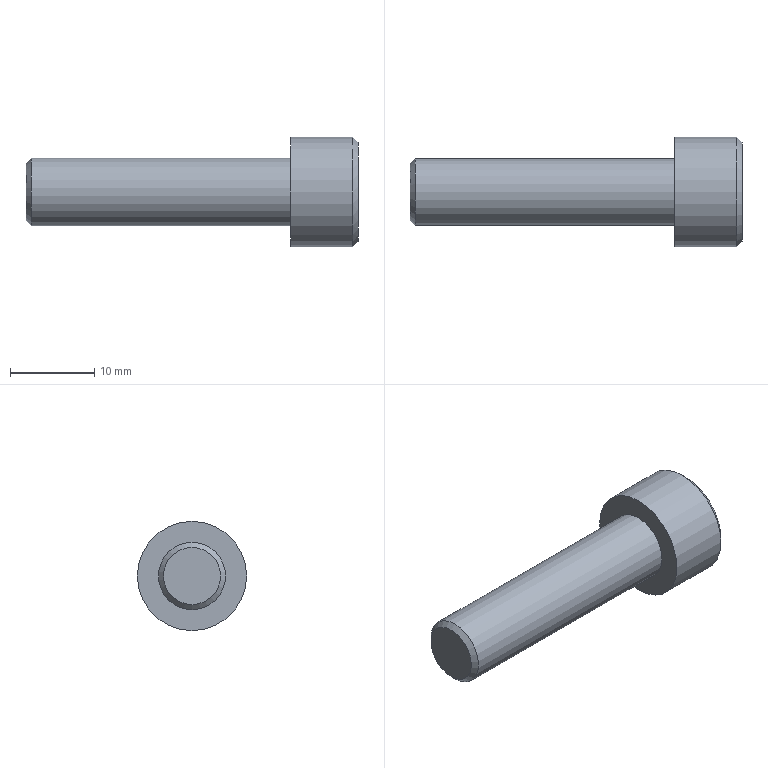Part | NX | features M8.00-60.00 2 | 1 solid | 14 faces | box 39.5 x 13 x 13 mm | volume 2474 mm3 | plane 10 | cylinder 2 | cone 2 | commonest cylinder face diameters 8 x1 13 x1
STEP:
#1=CARTESIAN_POINT('',(103.775,14.,24.349));
#2=VERTEX_POINT('',#1);
#3=CARTESIAN_POINT('',(103.775,14.,18.449));
#4=DIRECTION('',(1.,0.,0.));
#5=DIRECTION('',(0.,0.,1.));
#6=AXIS2_PLACEMENT_3D('',#3,#4,#5);
#7=CIRCLE('',#6,5.9);
#8=EDGE_CURVE('',#2,#2,#7,.T.);
#9=ORIENTED_EDGE('',*,*,#8,.T.);
#10=EDGE_LOOP('',(#9));
#11=FACE_BOUND('',#10,.T.);
#12=CARTESIAN_POINT('',(103.775,17.4,16.486));
#13=VERTEX_POINT('',#12);
#14=CARTESIAN_POINT('',(103.775,17.4,20.412));
#15=VERTEX_POINT('',#14);
#16=CARTESIAN_POINT('',(103.775,17.4,16.486));
#17=DIRECTION('',(0.,0.,1.));
#18=VECTOR('',#17,1000.);
#19=LINE('',#16,#18);
#20=EDGE_CURVE('',#13,#15,#19,.T.);
#21=ORIENTED_EDGE('',*,*,#20,.F.);
#22=CARTESIAN_POINT('',(103.775,14.,14.523));
#23=VERTEX_POINT('',#22);
#24=CARTESIAN_POINT('',(103.775,14.,14.523));
#25=DIRECTION('',(0.,0.866,0.5));
#26=VECTOR('',#25,1000.);
#27=LINE('',#24,#26);
#28=EDGE_CURVE('',#23,#13,#27,.T.);
#29=ORIENTED_EDGE('',*,*,#28,.F.);
#30=CARTESIAN_POINT('',(103.775,10.6,16.486));
#31=VERTEX_POINT('',#30);
#32=CARTESIAN_POINT('',(103.775,10.6,16.486));
#33=DIRECTION('',(0.,0.866,-0.5));
#34=VECTOR('',#33,1000.);
#35=LINE('',#32,#34);
#36=EDGE_CURVE('',#31,#23,#35,.T.);
#37=ORIENTED_EDGE('',*,*,#36,.F.);
#38=CARTESIAN_POINT('',(103.775,10.6,20.412));
#39=VERTEX_POINT('',#38);
#40=CARTESIAN_POINT('',(103.775,10.6,20.412));
#41=DIRECTION('',(0.,0.,-1.));
#42=VECTOR('',#41,1000.);
#43=LINE('',#40,#42);
#44=EDGE_CURVE('',#39,#31,#43,.T.);
#45=ORIENTED_EDGE('',*,*,#44,.F.);
#46=CARTESIAN_POINT('',(103.775,14.,22.375));
#47=VERTEX_POINT('',#46);
#48=CARTESIAN_POINT('',(103.775,14.,22.375));
#49=DIRECTION('',(0.,-0.866,-0.5));
#50=VECTOR('',#49,1000.);
#51=LINE('',#48,#50);
#52=EDGE_CURVE('',#47,#39,#51,.T.);
#53=ORIENTED_EDGE('',*,*,#52,.F.);
#54=CARTESIAN_POINT('',(103.775,17.4,20.412));
#55=DIRECTION('',(0.,-0.866,0.5));
#56=VECTOR('',#55,1000.);
#57=LINE('',#54,#56);
#58=EDGE_CURVE('',#15,#47,#57,.T.);
#59=ORIENTED_EDGE('',*,*,#58,.F.);
#60=EDGE_LOOP('',(#21,#29,#37,#45,#53,#59));
#61=FACE_BOUND('',#60,.T.);
#62=CARTESIAN_POINT('',(103.775,14.,18.449));
#63=DIRECTION('',(1.,0.,0.));
#64=DIRECTION('',(0.,0.,1.));
#65=AXIS2_PLACEMENT_3D('',#62,#63,#64);
#66=PLANE('',#65);
#67=ADVANCED_FACE('',(#11,#61),#66,.T.);
#68=CARTESIAN_POINT('',(95.775,14.,14.449));
#69=VERTEX_POINT('',#68);
#70=CARTESIAN_POINT('',(95.775,14.,18.449));
#71=DIRECTION('',(-1.,0.,0.));
#72=DIRECTION('',(0.,0.,-1.));
#73=AXIS2_PLACEMENT_3D('',#70,#71,#72);
#74=CIRCLE('',#73,4.);
#75=EDGE_CURVE('',#69,#69,#74,.T.);
#76=ORIENTED_EDGE('',*,*,#75,.F.);
#77=EDGE_LOOP('',(#76));
#78=FACE_BOUND('',#77,.T.);
#79=CARTESIAN_POINT('',(95.775,14.,24.949));
#80=VERTEX_POINT('',#79);
#81=CARTESIAN_POINT('',(95.775,14.,18.449));
#82=DIRECTION('',(1.,0.,0.));
#83=DIRECTION('',(0.,0.,1.));
#84=AXIS2_PLACEMENT_3D('',#81,#82,#83);
#85=CIRCLE('',#84,6.5);
#86=EDGE_CURVE('',#80,#80,#85,.T.);
#87=ORIENTED_EDGE('',*,*,#86,.F.);
#88=EDGE_LOOP('',(#87));
#89=FACE_BOUND('',#88,.T.);
#90=CARTESIAN_POINT('',(95.775,14.,18.449));
#91=DIRECTION('',(-1.,0.,0.));
#92=DIRECTION('',(0.,0.,-1.));
#93=AXIS2_PLACEMENT_3D('',#90,#91,#92);
#94=PLANE('',#93);
#95=ADVANCED_FACE('',(#78,#89),#94,.T.);
#96=CARTESIAN_POINT('',(103.175,14.,24.949));
#97=VERTEX_POINT('',#96);
#98=CARTESIAN_POINT('',(103.175,14.,18.449));
#99=DIRECTION('',(1.,0.,0.));
#100=DIRECTION('',(0.,0.,1.));
#101=AXIS2_PLACEMENT_3D('',#98,#99,#100);
#102=CIRCLE('',#101,6.5);
#103=EDGE_CURVE('',#97,#97,#102,.F.);
#104=ORIENTED_EDGE('',*,*,#103,.T.);
#105=EDGE_LOOP('',(#104));
#106=FACE_BOUND('',#105,.T.);
#107=ORIENTED_EDGE('',*,*,#86,.T.);
#108=EDGE_LOOP('',(#107));
#109=FACE_BOUND('',#108,.T.);
#110=CARTESIAN_POINT('',(95.775,14.,18.449));
#111=DIRECTION('',(1.,0.,0.));
#112=DIRECTION('',(0.,0.,1.));
#113=AXIS2_PLACEMENT_3D('',#110,#111,#112);
#114=CYLINDRICAL_SURFACE('',#113,6.5);
#115=ADVANCED_FACE('',(#106,#109),#114,.T.);
#116=CARTESIAN_POINT('',(64.275,14.,15.049));
#117=VERTEX_POINT('',#116);
#118=CARTESIAN_POINT('',(64.275,14.,18.449));
#119=DIRECTION('',(-1.,0.,0.));
#120=DIRECTION('',(0.,0.,-1.));
#121=AXIS2_PLACEMENT_3D('',#118,#119,#120);
#122=CIRCLE('',#121,3.4);
#123=EDGE_CURVE('',#117,#117,#122,.T.);
#124=ORIENTED_EDGE('',*,*,#123,.T.);
#125=EDGE_LOOP('',(#124));
#126=FACE_BOUND('',#125,.T.);
#127=CARTESIAN_POINT('',(64.275,14.,18.449));
#128=DIRECTION('',(-1.,0.,0.));
#129=DIRECTION('',(0.,0.,-1.));
#130=AXIS2_PLACEMENT_3D('',#127,#128,#129);
#131=PLANE('',#130);
#132=ADVANCED_FACE('',(#126),#131,.T.);
#133=CARTESIAN_POINT('',(64.875,14.,14.449));
#134=VERTEX_POINT('',#133);
#135=CARTESIAN_POINT('',(64.875,14.,18.449));
#136=DIRECTION('',(-1.,0.,0.));
#137=DIRECTION('',(0.,0.,-1.));
#138=AXIS2_PLACEMENT_3D('',#135,#136,#137);
#139=CIRCLE('',#138,4.);
#140=EDGE_CURVE('',#134,#134,#139,.F.);
#141=ORIENTED_EDGE('',*,*,#140,.T.);
#142=EDGE_LOOP('',(#141));
#143=FACE_BOUND('',#142,.T.);
#144=ORIENTED_EDGE('',*,*,#75,.T.);
#145=EDGE_LOOP('',(#144));
#146=FACE_BOUND('',#145,.T.);
#147=CARTESIAN_POINT('',(116.275,14.,18.449));
#148=DIRECTION('',(-1.,0.,0.));
#149=DIRECTION('',(0.,0.,-1.));
#150=AXIS2_PLACEMENT_3D('',#147,#148,#149);
#151=CYLINDRICAL_SURFACE('',#150,4.);
#152=ADVANCED_FACE('',(#143,#146),#151,.T.);
#153=ORIENTED_EDGE('',*,*,#58,.T.);
#154=CARTESIAN_POINT('',(99.775,14.,22.375));
#155=VERTEX_POINT('',#154);
#156=CARTESIAN_POINT('',(99.775,14.,22.375));
#157=DIRECTION('',(1.,0.,0.));
#158=VECTOR('',#157,1000.);
#159=LINE('',#156,#158);
#160=EDGE_CURVE('',#47,#155,#159,.F.);
#161=ORIENTED_EDGE('',*,*,#160,.T.);
#162=CARTESIAN_POINT('',(99.775,17.4,20.412));
#163=VERTEX_POINT('',#162);
#164=CARTESIAN_POINT('',(99.775,17.4,20.412));
#165=DIRECTION('',(0.,-0.866,0.5));
#166=VECTOR('',#165,1000.);
#167=LINE('',#164,#166);
#168=EDGE_CURVE('',#155,#163,#167,.F.);
#169=ORIENTED_EDGE('',*,*,#168,.T.);
#170=CARTESIAN_POINT('',(99.775,17.4,20.412));
#171=DIRECTION('',(1.,0.,0.));
#172=VECTOR('',#171,1000.);
#173=LINE('',#170,#172);
#174=EDGE_CURVE('',#15,#163,#173,.F.);
#175=ORIENTED_EDGE('',*,*,#174,.F.);
#176=EDGE_LOOP('',(#153,#161,#169,#175));
#177=FACE_BOUND('',#176,.T.);
#178=CARTESIAN_POINT('',(101.775,15.7,21.393));
#179=DIRECTION('',(0.,0.5,0.866));
#180=DIRECTION('',(0.,-0.866,0.5));
#181=AXIS2_PLACEMENT_3D('',#178,#179,#180);
#182=PLANE('',#181);
#183=ADVANCED_FACE('',(#177),#182,.F.);
#184=ORIENTED_EDGE('',*,*,#20,.T.);
#185=ORIENTED_EDGE('',*,*,#174,.T.);
#186=CARTESIAN_POINT('',(99.775,17.4,16.486));
#187=VERTEX_POINT('',#186);
#188=CARTESIAN_POINT('',(99.775,17.4,16.486));
#189=DIRECTION('',(0.,0.,1.));
#190=VECTOR('',#189,1000.);
#191=LINE('',#188,#190);
#192=EDGE_CURVE('',#163,#187,#191,.F.);
#193=ORIENTED_EDGE('',*,*,#192,.T.);
#194=CARTESIAN_POINT('',(99.775,17.4,16.486));
#195=DIRECTION('',(1.,0.,0.));
#196=VECTOR('',#195,1000.);
#197=LINE('',#194,#196);
#198=EDGE_CURVE('',#13,#187,#197,.F.);
#199=ORIENTED_EDGE('',*,*,#198,.F.);
#200=EDGE_LOOP('',(#184,#185,#193,#199));
#201=FACE_BOUND('',#200,.T.);
#202=CARTESIAN_POINT('',(101.775,17.4,18.449));
#203=DIRECTION('',(0.,1.,0.));
#204=DIRECTION('',(1.,0.,0.));
#205=AXIS2_PLACEMENT_3D('',#202,#203,#204);
#206=PLANE('',#205);
#207=ADVANCED_FACE('',(#201),#206,.F.);
#208=ORIENTED_EDGE('',*,*,#28,.T.);
#209=ORIENTED_EDGE('',*,*,#198,.T.);
#210=CARTESIAN_POINT('',(99.775,14.,14.523));
#211=VERTEX_POINT('',#210);
#212=CARTESIAN_POINT('',(99.775,14.,14.523));
#213=DIRECTION('',(0.,0.866,0.5));
#214=VECTOR('',#213,1000.);
#215=LINE('',#212,#214);
#216=EDGE_CURVE('',#187,#211,#215,.F.);
#217=ORIENTED_EDGE('',*,*,#216,.T.);
#218=CARTESIAN_POINT('',(99.775,14.,14.523));
#219=DIRECTION('',(1.,0.,0.));
#220=VECTOR('',#219,1000.);
#221=LINE('',#218,#220);
#222=EDGE_CURVE('',#23,#211,#221,.F.);
#223=ORIENTED_EDGE('',*,*,#222,.F.);
#224=EDGE_LOOP('',(#208,#209,#217,#223));
#225=FACE_BOUND('',#224,.T.);
#226=CARTESIAN_POINT('',(101.775,15.7,15.504));
#227=DIRECTION('',(0.,0.5,-0.866));
#228=DIRECTION('',(0.,0.866,0.5));
#229=AXIS2_PLACEMENT_3D('',#226,#227,#228);
#230=PLANE('',#229);
#231=ADVANCED_FACE('',(#225),#230,.F.);
#232=ORIENTED_EDGE('',*,*,#36,.T.);
#233=ORIENTED_EDGE('',*,*,#222,.T.);
#234=CARTESIAN_POINT('',(99.775,10.6,16.486));
#235=VERTEX_POINT('',#234);
#236=CARTESIAN_POINT('',(99.775,10.6,16.486));
#237=DIRECTION('',(0.,0.866,-0.5));
#238=VECTOR('',#237,1000.);
#239=LINE('',#236,#238);
#240=EDGE_CURVE('',#211,#235,#239,.F.);
#241=ORIENTED_EDGE('',*,*,#240,.T.);
#242=CARTESIAN_POINT('',(99.775,10.6,16.486));
#243=DIRECTION('',(1.,0.,0.));
#244=VECTOR('',#243,1000.);
#245=LINE('',#242,#244);
#246=EDGE_CURVE('',#31,#235,#245,.F.);
#247=ORIENTED_EDGE('',*,*,#246,.F.);
#248=EDGE_LOOP('',(#232,#233,#241,#247));
#249=FACE_BOUND('',#248,.T.);
#250=CARTESIAN_POINT('',(101.775,12.3,15.504));
#251=DIRECTION('',(0.,-0.5,-0.866));
#252=DIRECTION('',(0.,0.866,-0.5));
#253=AXIS2_PLACEMENT_3D('',#250,#251,#252);
#254=PLANE('',#253);
#255=ADVANCED_FACE('',(#249),#254,.F.);
#256=ORIENTED_EDGE('',*,*,#44,.T.);
#257=ORIENTED_EDGE('',*,*,#246,.T.);
#258=CARTESIAN_POINT('',(99.775,10.6,20.412));
#259=VERTEX_POINT('',#258);
#260=CARTESIAN_POINT('',(99.775,10.6,20.412));
#261=DIRECTION('',(0.,0.,-1.));
#262=VECTOR('',#261,1000.);
#263=LINE('',#260,#262);
#264=EDGE_CURVE('',#235,#259,#263,.F.);
#265=ORIENTED_EDGE('',*,*,#264,.T.);
#266=CARTESIAN_POINT('',(99.775,10.6,20.412));
#267=DIRECTION('',(1.,0.,0.));
#268=VECTOR('',#267,1000.);
#269=LINE('',#266,#268);
#270=EDGE_CURVE('',#39,#259,#269,.F.);
#271=ORIENTED_EDGE('',*,*,#270,.F.);
#272=EDGE_LOOP('',(#256,#257,#265,#271));
#273=FACE_BOUND('',#272,.T.);
#274=CARTESIAN_POINT('',(101.775,10.6,18.449));
#275=DIRECTION('',(0.,-1.,0.));
#276=DIRECTION('',(-1.,0.,0.));
#277=AXIS2_PLACEMENT_3D('',#274,#275,#276);
#278=PLANE('',#277);
#279=ADVANCED_FACE('',(#273),#278,.F.);
#280=ORIENTED_EDGE('',*,*,#52,.T.);
#281=ORIENTED_EDGE('',*,*,#270,.T.);
#282=CARTESIAN_POINT('',(99.775,14.,22.375));
#283=DIRECTION('',(0.,-0.866,-0.5));
#284=VECTOR('',#283,1000.);
#285=LINE('',#282,#284);
#286=EDGE_CURVE('',#259,#155,#285,.F.);
#287=ORIENTED_EDGE('',*,*,#286,.T.);
#288=ORIENTED_EDGE('',*,*,#160,.F.);
#289=EDGE_LOOP('',(#280,#281,#287,#288));
#290=FACE_BOUND('',#289,.T.);
#291=CARTESIAN_POINT('',(101.775,12.3,21.393));
#292=DIRECTION('',(0.,-0.5,0.866));
#293=DIRECTION('',(0.,-0.866,-0.5));
#294=AXIS2_PLACEMENT_3D('',#291,#292,#293);
#295=PLANE('',#294);
#296=ADVANCED_FACE('',(#290),#295,.F.);
#297=ORIENTED_EDGE('',*,*,#286,.F.);
#298=ORIENTED_EDGE('',*,*,#264,.F.);
#299=ORIENTED_EDGE('',*,*,#240,.F.);
#300=ORIENTED_EDGE('',*,*,#216,.F.);
#301=ORIENTED_EDGE('',*,*,#192,.F.);
#302=ORIENTED_EDGE('',*,*,#168,.F.);
#303=EDGE_LOOP('',(#297,#298,#299,#300,#301,#302));
#304=FACE_BOUND('',#303,.T.);
#305=CARTESIAN_POINT('',(99.775,14.,18.449));
#306=DIRECTION('',(-1.,0.,0.));
#307=DIRECTION('',(0.,0.,-1.));
#308=AXIS2_PLACEMENT_3D('',#305,#306,#307);
#309=PLANE('',#308);
#310=ADVANCED_FACE('',(#304),#309,.F.);
#311=ORIENTED_EDGE('',*,*,#123,.F.);
#312=EDGE_LOOP('',(#311));
#313=FACE_BOUND('',#312,.T.);
#314=ORIENTED_EDGE('',*,*,#140,.F.);
#315=EDGE_LOOP('',(#314));
#316=FACE_BOUND('',#315,.T.);
#317=CARTESIAN_POINT('',(64.875,14.,18.449));
#318=DIRECTION('',(1.,0.,0.));
#319=DIRECTION('',(0.,0.,1.));
#320=AXIS2_PLACEMENT_3D('',#317,#318,#319);
#321=CONICAL_SURFACE('',#320,4.,0.7854);
#322=ADVANCED_FACE('',(#313,#316),#321,.T.);
#323=ORIENTED_EDGE('',*,*,#8,.F.);
#324=EDGE_LOOP('',(#323));
#325=FACE_BOUND('',#324,.T.);
#326=ORIENTED_EDGE('',*,*,#103,.F.);
#327=EDGE_LOOP('',(#326));
#328=FACE_BOUND('',#327,.T.);
#329=CARTESIAN_POINT('',(103.175,14.,18.449));
#330=DIRECTION('',(-1.,0.,0.));
#331=DIRECTION('',(0.,0.,-1.));
#332=AXIS2_PLACEMENT_3D('',#329,#330,#331);
#333=CONICAL_SURFACE('',#332,6.5,0.7854);
#334=ADVANCED_FACE('',(#325,#328),#333,.T.);
#335=CLOSED_SHELL('',(#67,#95,#115,#132,#152,#183,#207,#231,#255,#279,#296,#310,#322,#334));
#336=MANIFOLD_SOLID_BREP('',#335);
#337=(LENGTH_UNIT()NAMED_UNIT(*)SI_UNIT(.MILLI.,.METRE.));
#338=UNCERTAINTY_MEASURE_WITH_UNIT(LENGTH_MEASURE(0.00001),#337,'','');
#339=(NAMED_UNIT(*)PLANE_ANGLE_UNIT()SI_UNIT($,.RADIAN.));
#340=(NAMED_UNIT(*)SI_UNIT($,.STERADIAN.)SOLID_ANGLE_UNIT());
#341=(GEOMETRIC_REPRESENTATION_CONTEXT(3)GLOBAL_UNCERTAINTY_ASSIGNED_CONTEXT((#338))GLOBAL_UNIT_ASSIGNED_CONTEXT((#337,#339,#340))REPRESENTATION_CONTEXT('',''));
#342=ADVANCED_BREP_SHAPE_REPRESENTATION('',(#336),#341);